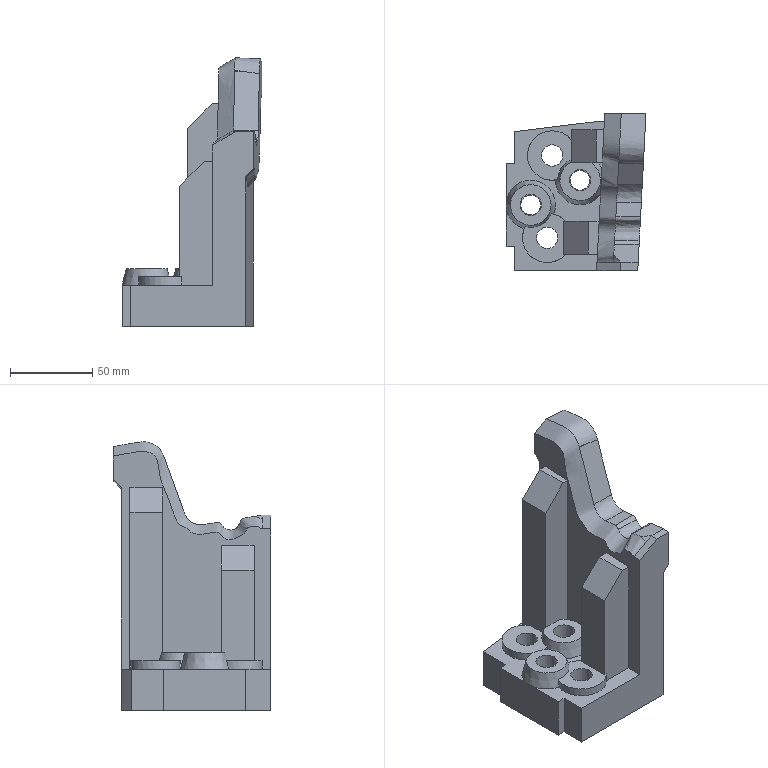Part | NX | features solid 2 | 1 solid | 61 faces | box 85 x 95.494 x 163.086 mm | volume 439456 mm3 | plane 33 | spline 17 | cylinder 9 | cone 2 | commonest cylinder face diameters 13 x4 30 x3 12 x2